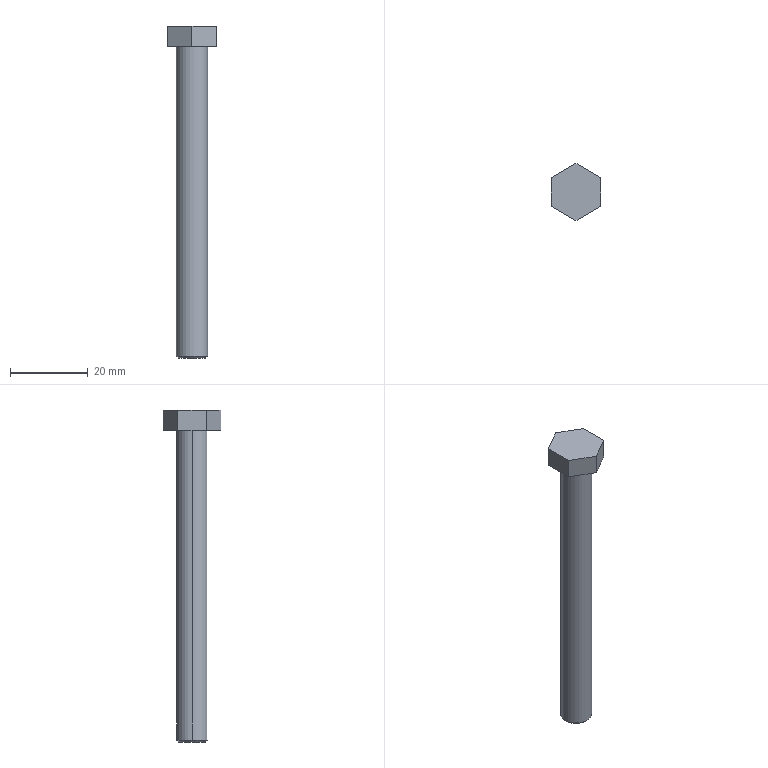Part | STEP file | Bulong M8_8F | 1 solid | 13 faces | box 12.73 x 14.699 x 85.15 mm | volume 4741 mm3 | plane 9 | cone 2 | cylinder 2 | commonest cylinder face diameters 8 x2
STEP:
#1=CARTESIAN_POINT('',(0.,0.,0.));
#2=DIRECTION('',(0.,0.,1.));
#3=DIRECTION('',(1.,0.,0.));
#4=AXIS2_PLACEMENT_3D('',#1,#2,#3);
#5=CARTESIAN_POINT('',(-3.5,0.,-80.));
#6=VERTEX_POINT('',#5);
#7=CARTESIAN_POINT('',(3.5,0.,-80.));
#8=VERTEX_POINT('',#7);
#9=CARTESIAN_POINT('',(0.,0.,-80.));
#10=DIRECTION('',(0.,0.,-1.));
#11=DIRECTION('',(-1.,0.,0.));
#12=AXIS2_PLACEMENT_3D('',#9,#10,#11);
#13=CIRCLE('',#12,3.5);
#14=CARTESIAN_POINT('',(0.,0.,-80.));
#15=DIRECTION('',(0.,0.,1.));
#16=DIRECTION('',(1.,0.,0.));
#17=AXIS2_PLACEMENT_3D('',#14,#15,#16);
#18=CONICAL_SURFACE('',#17,3.5,0.7854);
#19=CARTESIAN_POINT('',(3.142,0.));
#20=DIRECTION('',(-1.,0.));
#21=VECTOR('',#20,1.);
#22=LINE('',#19,#21);
#23=(GEOMETRIC_REPRESENTATION_CONTEXT(2)PARAMETRIC_REPRESENTATION_CONTEXT()REPRESENTATION_CONTEXT('',''));
#24=DEFINITIONAL_REPRESENTATION('',(#22),#23);
#25=PCURVE('',#18,#24);
#26=CARTESIAN_POINT('',(0.,0.,-80.));
#27=DIRECTION('',(0.,0.,-1.));
#28=DIRECTION('',(-1.,0.,0.));
#29=AXIS2_PLACEMENT_3D('',#26,#27,#28);
#30=PLANE('',#29);
#31=CARTESIAN_POINT('',(0.,0.));
#32=DIRECTION('',(1.,0.));
#33=AXIS2_PLACEMENT_2D('',#31,#32);
#34=CIRCLE('',#33,3.5);
#35=(GEOMETRIC_REPRESENTATION_CONTEXT(2)PARAMETRIC_REPRESENTATION_CONTEXT()REPRESENTATION_CONTEXT('',''));
#36=DEFINITIONAL_REPRESENTATION('',(#34),#35);
#37=PCURVE('',#30,#36);
#38=SURFACE_CURVE('',#13,(#25,#37),.PCURVE_S1.);
#39=EDGE_CURVE('',#6,#8,#38,.T.);
#40=ORIENTED_EDGE('',*,*,#39,.F.);
#41=CARTESIAN_POINT('',(-4.,0.,-79.5));
#42=VERTEX_POINT('',#41);
#43=CARTESIAN_POINT('',(-3.5,0.,-80.));
#44=DIRECTION('',(-0.7071,0.,0.7071));
#45=VECTOR('',#44,1.);
#46=LINE('',#43,#45);
#47=CARTESIAN_POINT('',(3.142,0.));
#48=DIRECTION('',(0.,1.));
#49=VECTOR('',#48,1.);
#50=LINE('',#47,#49);
#51=(GEOMETRIC_REPRESENTATION_CONTEXT(2)PARAMETRIC_REPRESENTATION_CONTEXT()REPRESENTATION_CONTEXT('',''));
#52=DEFINITIONAL_REPRESENTATION('',(#50),#51);
#53=PCURVE('',#18,#52);
#54=CARTESIAN_POINT('',(0.,0.,-80.));
#55=DIRECTION('',(0.,0.,1.));
#56=DIRECTION('',(1.,0.,0.));
#57=AXIS2_PLACEMENT_3D('',#54,#55,#56);
#58=CONICAL_SURFACE('',#57,3.5,0.7854);
#59=CARTESIAN_POINT('',(3.142,0.));
#60=DIRECTION('',(0.,1.));
#61=VECTOR('',#60,1.);
#62=LINE('',#59,#61);
#63=(GEOMETRIC_REPRESENTATION_CONTEXT(2)PARAMETRIC_REPRESENTATION_CONTEXT()REPRESENTATION_CONTEXT('',''));
#64=DEFINITIONAL_REPRESENTATION('',(#62),#63);
#65=PCURVE('',#58,#64);
#66=SURFACE_CURVE('',#46,(#53,#65),.PCURVE_S1.);
#67=EDGE_CURVE('',#6,#42,#66,.T.);
#68=ORIENTED_EDGE('',*,*,#67,.T.);
#69=CARTESIAN_POINT('',(4.,0.,-79.5));
#70=VERTEX_POINT('',#69);
#71=CARTESIAN_POINT('',(0.,0.,-79.5));
#72=DIRECTION('',(0.,0.,1.));
#73=DIRECTION('',(-1.,0.,0.));
#74=AXIS2_PLACEMENT_3D('',#71,#72,#73);
#75=CIRCLE('',#74,4.);
#76=CARTESIAN_POINT('',(-3.142,0.5));
#77=DIRECTION('',(1.,0.));
#78=VECTOR('',#77,1.);
#79=LINE('',#76,#78);
#80=(GEOMETRIC_REPRESENTATION_CONTEXT(2)PARAMETRIC_REPRESENTATION_CONTEXT()REPRESENTATION_CONTEXT('',''));
#81=DEFINITIONAL_REPRESENTATION('',(#79),#80);
#82=PCURVE('',#18,#81);
#83=CARTESIAN_POINT('',(0.,0.,-80.));
#84=DIRECTION('',(0.,0.,1.));
#85=DIRECTION('',(1.,0.,0.));
#86=AXIS2_PLACEMENT_3D('',#83,#84,#85);
#87=CYLINDRICAL_SURFACE('',#86,4.);
#88=CARTESIAN_POINT('',(-3.142,0.5));
#89=DIRECTION('',(1.,0.));
#90=VECTOR('',#89,1.);
#91=LINE('',#88,#90);
#92=(GEOMETRIC_REPRESENTATION_CONTEXT(2)PARAMETRIC_REPRESENTATION_CONTEXT()REPRESENTATION_CONTEXT('',''));
#93=DEFINITIONAL_REPRESENTATION('',(#91),#92);
#94=PCURVE('',#87,#93);
#95=SURFACE_CURVE('',#75,(#82,#94),.PCURVE_S1.);
#96=EDGE_CURVE('',#70,#42,#95,.T.);
#97=ORIENTED_EDGE('',*,*,#96,.F.);
#98=CARTESIAN_POINT('',(3.5,0.,-80.));
#99=DIRECTION('',(0.7071,0.,0.7071));
#100=VECTOR('',#99,1.);
#101=LINE('',#98,#100);
#102=CARTESIAN_POINT('',(0.,0.));
#103=DIRECTION('',(0.,1.));
#104=VECTOR('',#103,1.);
#105=LINE('',#102,#104);
#106=(GEOMETRIC_REPRESENTATION_CONTEXT(2)PARAMETRIC_REPRESENTATION_CONTEXT()REPRESENTATION_CONTEXT('',''));
#107=DEFINITIONAL_REPRESENTATION('',(#105),#106);
#108=PCURVE('',#18,#107);
#109=CARTESIAN_POINT('',(6.283,0.));
#110=DIRECTION('',(0.,1.));
#111=VECTOR('',#110,1.);
#112=LINE('',#109,#111);
#113=(GEOMETRIC_REPRESENTATION_CONTEXT(2)PARAMETRIC_REPRESENTATION_CONTEXT()REPRESENTATION_CONTEXT('',''));
#114=DEFINITIONAL_REPRESENTATION('',(#112),#113);
#115=PCURVE('',#58,#114);
#116=SURFACE_CURVE('',#101,(#108,#115),.PCURVE_S1.);
#117=EDGE_CURVE('',#8,#70,#116,.T.);
#118=ORIENTED_EDGE('',*,*,#117,.F.);
#119=EDGE_LOOP('',(#40,#68,#97,#118));
#120=FACE_BOUND('',#119,.T.);
#121=ADVANCED_FACE('',(#120),#18,.T.);
#122=ORIENTED_EDGE('',*,*,#96,.T.);
#123=CARTESIAN_POINT('',(-4.,0.,0.));
#124=VERTEX_POINT('',#123);
#125=CARTESIAN_POINT('',(-4.,0.,-80.));
#126=DIRECTION('',(0.,0.,1.));
#127=VECTOR('',#126,1.);
#128=LINE('',#125,#127);
#129=CARTESIAN_POINT('',(3.142,0.));
#130=DIRECTION('',(0.,1.));
#131=VECTOR('',#130,1.);
#132=LINE('',#129,#131);
#133=(GEOMETRIC_REPRESENTATION_CONTEXT(2)PARAMETRIC_REPRESENTATION_CONTEXT()REPRESENTATION_CONTEXT('',''));
#134=DEFINITIONAL_REPRESENTATION('',(#132),#133);
#135=PCURVE('',#87,#134);
#136=CARTESIAN_POINT('',(0.,0.,-80.));
#137=DIRECTION('',(0.,0.,1.));
#138=DIRECTION('',(1.,0.,0.));
#139=AXIS2_PLACEMENT_3D('',#136,#137,#138);
#140=CYLINDRICAL_SURFACE('',#139,4.);
#141=CARTESIAN_POINT('',(3.142,0.));
#142=DIRECTION('',(0.,1.));
#143=VECTOR('',#142,1.);
#144=LINE('',#141,#143);
#145=(GEOMETRIC_REPRESENTATION_CONTEXT(2)PARAMETRIC_REPRESENTATION_CONTEXT()REPRESENTATION_CONTEXT('',''));
#146=DEFINITIONAL_REPRESENTATION('',(#144),#145);
#147=PCURVE('',#140,#146);
#148=SURFACE_CURVE('',#128,(#135,#147),.PCURVE_S1.);
#149=EDGE_CURVE('',#42,#124,#148,.T.);
#150=ORIENTED_EDGE('',*,*,#149,.T.);
#151=CARTESIAN_POINT('',(4.,0.,0.));
#152=VERTEX_POINT('',#151);
#153=CARTESIAN_POINT('',(0.,0.,0.));
#154=DIRECTION('',(0.,0.,-1.));
#155=DIRECTION('',(1.,0.,0.));
#156=AXIS2_PLACEMENT_3D('',#153,#154,#155);
#157=CIRCLE('',#156,4.);
#158=CARTESIAN_POINT('',(6.283,80.));
#159=DIRECTION('',(-1.,0.));
#160=VECTOR('',#159,1.);
#161=LINE('',#158,#160);
#162=(GEOMETRIC_REPRESENTATION_CONTEXT(2)PARAMETRIC_REPRESENTATION_CONTEXT()REPRESENTATION_CONTEXT('',''));
#163=DEFINITIONAL_REPRESENTATION('',(#161),#162);
#164=PCURVE('',#87,#163);
#165=CARTESIAN_POINT('',(0.,0.,0.));
#166=DIRECTION('',(0.,0.,1.));
#167=DIRECTION('',(1.,0.,0.));
#168=AXIS2_PLACEMENT_3D('',#165,#166,#167);
#169=PLANE('',#168);
#170=CARTESIAN_POINT('',(4.,0.));
#171=CARTESIAN_POINT('',(4.,-6.928));
#172=CARTESIAN_POINT('',(-2.,-3.464));
#173=CARTESIAN_POINT('',(-8.,0.));
#174=CARTESIAN_POINT('',(-2.,3.464));
#175=CARTESIAN_POINT('',(4.,6.928));
#176=CARTESIAN_POINT('',(4.,0.));
#177=(BOUNDED_CURVE()B_SPLINE_CURVE(2,(#170,#171,#172,#173,#174,#175,#176),.UNSPECIFIED.,.T.,.F.)B_SPLINE_CURVE_WITH_KNOTS((1,2,2,2,2,1),(-2.094,0.,2.094,4.189,6.283,8.378),.UNSPECIFIED.)CURVE()GEOMETRIC_REPRESENTATION_ITEM()RATIONAL_B_SPLINE_CURVE((1.,0.5,1.,0.5,1.,0.5,1.))REPRESENTATION_ITEM(''));
#178=(GEOMETRIC_REPRESENTATION_CONTEXT(2)PARAMETRIC_REPRESENTATION_CONTEXT()REPRESENTATION_CONTEXT('',''));
#179=DEFINITIONAL_REPRESENTATION('',(#177),#178);
#180=PCURVE('',#169,#179);
#181=SURFACE_CURVE('',#157,(#164,#180),.PCURVE_S1.);
#182=EDGE_CURVE('',#124,#152,#181,.T.);
#183=ORIENTED_EDGE('',*,*,#182,.T.);
#184=CARTESIAN_POINT('',(4.,0.,-80.));
#185=DIRECTION('',(0.,0.,1.));
#186=VECTOR('',#185,1.);
#187=LINE('',#184,#186);
#188=CARTESIAN_POINT('',(0.,0.));
#189=DIRECTION('',(0.,1.));
#190=VECTOR('',#189,1.);
#191=LINE('',#188,#190);
#192=(GEOMETRIC_REPRESENTATION_CONTEXT(2)PARAMETRIC_REPRESENTATION_CONTEXT()REPRESENTATION_CONTEXT('',''));
#193=DEFINITIONAL_REPRESENTATION('',(#191),#192);
#194=PCURVE('',#87,#193);
#195=CARTESIAN_POINT('',(6.283,0.));
#196=DIRECTION('',(0.,1.));
#197=VECTOR('',#196,1.);
#198=LINE('',#195,#197);
#199=(GEOMETRIC_REPRESENTATION_CONTEXT(2)PARAMETRIC_REPRESENTATION_CONTEXT()REPRESENTATION_CONTEXT('',''));
#200=DEFINITIONAL_REPRESENTATION('',(#198),#199);
#201=PCURVE('',#140,#200);
#202=SURFACE_CURVE('',#187,(#194,#201),.PCURVE_S1.);
#203=EDGE_CURVE('',#70,#152,#202,.T.);
#204=ORIENTED_EDGE('',*,*,#203,.F.);
#205=EDGE_LOOP('',(#122,#150,#183,#204));
#206=FACE_BOUND('',#205,.T.);
#207=ADVANCED_FACE('',(#206),#87,.T.);
#208=CARTESIAN_POINT('',(6.365,3.675,0.));
#209=VERTEX_POINT('',#208);
#210=CARTESIAN_POINT('',(0.,7.35,0.));
#211=VERTEX_POINT('',#210);
#212=CARTESIAN_POINT('',(6.365,3.675,0.));
#213=DIRECTION('',(-0.866,0.5,0.));
#214=VECTOR('',#213,1.);
#215=LINE('',#212,#214);
#216=CARTESIAN_POINT('',(6.365,3.675));
#217=DIRECTION('',(-0.866,0.5));
#218=VECTOR('',#217,1.);
#219=LINE('',#216,#218);
#220=(GEOMETRIC_REPRESENTATION_CONTEXT(2)PARAMETRIC_REPRESENTATION_CONTEXT()REPRESENTATION_CONTEXT('',''));
#221=DEFINITIONAL_REPRESENTATION('',(#219),#220);
#222=PCURVE('',#169,#221);
#223=CARTESIAN_POINT('',(6.365,3.675,5.15));
#224=DIRECTION('',(-0.5,-0.866,0.));
#225=DIRECTION('',(0.866,-0.5,0.));
#226=AXIS2_PLACEMENT_3D('',#223,#224,#225);
#227=PLANE('',#226);
#228=CARTESIAN_POINT('',(0.,-5.15));
#229=DIRECTION('',(-1.,0.));
#230=VECTOR('',#229,1.);
#231=LINE('',#228,#230);
#232=(GEOMETRIC_REPRESENTATION_CONTEXT(2)PARAMETRIC_REPRESENTATION_CONTEXT()REPRESENTATION_CONTEXT('',''));
#233=DEFINITIONAL_REPRESENTATION('',(#231),#232);
#234=PCURVE('',#227,#233);
#235=SURFACE_CURVE('',#215,(#222,#234),.PCURVE_S1.);
#236=EDGE_CURVE('',#209,#211,#235,.T.);
#237=ORIENTED_EDGE('',*,*,#236,.F.);
#238=CARTESIAN_POINT('',(6.365,-3.675,0.));
#239=VERTEX_POINT('',#238);
#240=CARTESIAN_POINT('',(6.365,-3.675,0.));
#241=DIRECTION('',(0.,1.,0.));
#242=VECTOR('',#241,1.);
#243=LINE('',#240,#242);
#244=CARTESIAN_POINT('',(6.365,-3.675));
#245=DIRECTION('',(0.,1.));
#246=VECTOR('',#245,1.);
#247=LINE('',#244,#246);
#248=(GEOMETRIC_REPRESENTATION_CONTEXT(2)PARAMETRIC_REPRESENTATION_CONTEXT()REPRESENTATION_CONTEXT('',''));
#249=DEFINITIONAL_REPRESENTATION('',(#247),#248);
#250=PCURVE('',#169,#249);
#251=CARTESIAN_POINT('',(6.365,-3.675,5.15));
#252=DIRECTION('',(-1.,0.,0.));
#253=DIRECTION('',(0.,-1.,0.));
#254=AXIS2_PLACEMENT_3D('',#251,#252,#253);
#255=PLANE('',#254);
#256=CARTESIAN_POINT('',(0.,-5.15));
#257=DIRECTION('',(-1.,0.));
#258=VECTOR('',#257,1.);
#259=LINE('',#256,#258);
#260=(GEOMETRIC_REPRESENTATION_CONTEXT(2)PARAMETRIC_REPRESENTATION_CONTEXT()REPRESENTATION_CONTEXT('',''));
#261=DEFINITIONAL_REPRESENTATION('',(#259),#260);
#262=PCURVE('',#255,#261);
#263=SURFACE_CURVE('',#243,(#250,#262),.PCURVE_S1.);
#264=EDGE_CURVE('',#239,#209,#263,.T.);
#265=ORIENTED_EDGE('',*,*,#264,.F.);
#266=CARTESIAN_POINT('',(0.,-7.35,0.));
#267=VERTEX_POINT('',#266);
#268=CARTESIAN_POINT('',(0.,-7.35,0.));
#269=DIRECTION('',(0.866,0.5,0.));
#270=VECTOR('',#269,1.);
#271=LINE('',#268,#270);
#272=CARTESIAN_POINT('',(0.,-7.35));
#273=DIRECTION('',(0.866,0.5));
#274=VECTOR('',#273,1.);
#275=LINE('',#272,#274);
#276=(GEOMETRIC_REPRESENTATION_CONTEXT(2)PARAMETRIC_REPRESENTATION_CONTEXT()REPRESENTATION_CONTEXT('',''));
#277=DEFINITIONAL_REPRESENTATION('',(#275),#276);
#278=PCURVE('',#169,#277);
#279=CARTESIAN_POINT('',(0.,-7.35,5.15));
#280=DIRECTION('',(-0.5,0.866,0.));
#281=DIRECTION('',(-0.866,-0.5,0.));
#282=AXIS2_PLACEMENT_3D('',#279,#280,#281);
#283=PLANE('',#282);
#284=CARTESIAN_POINT('',(0.,-5.15));
#285=DIRECTION('',(-1.,0.));
#286=VECTOR('',#285,1.);
#287=LINE('',#284,#286);
#288=(GEOMETRIC_REPRESENTATION_CONTEXT(2)PARAMETRIC_REPRESENTATION_CONTEXT()REPRESENTATION_CONTEXT('',''));
#289=DEFINITIONAL_REPRESENTATION('',(#287),#288);
#290=PCURVE('',#283,#289);
#291=SURFACE_CURVE('',#271,(#278,#290),.PCURVE_S1.);
#292=EDGE_CURVE('',#267,#239,#291,.T.);
#293=ORIENTED_EDGE('',*,*,#292,.F.);
#294=CARTESIAN_POINT('',(-6.365,-3.675,0.));
#295=VERTEX_POINT('',#294);
#296=CARTESIAN_POINT('',(-6.365,-3.675,0.));
#297=DIRECTION('',(0.866,-0.5,0.));
#298=VECTOR('',#297,1.);
#299=LINE('',#296,#298);
#300=CARTESIAN_POINT('',(-6.365,-3.675));
#301=DIRECTION('',(0.866,-0.5));
#302=VECTOR('',#301,1.);
#303=LINE('',#300,#302);
#304=(GEOMETRIC_REPRESENTATION_CONTEXT(2)PARAMETRIC_REPRESENTATION_CONTEXT()REPRESENTATION_CONTEXT('',''));
#305=DEFINITIONAL_REPRESENTATION('',(#303),#304);
#306=PCURVE('',#169,#305);
#307=CARTESIAN_POINT('',(-6.365,-3.675,5.15));
#308=DIRECTION('',(0.5,0.866,0.));
#309=DIRECTION('',(-0.866,0.5,0.));
#310=AXIS2_PLACEMENT_3D('',#307,#308,#309);
#311=PLANE('',#310);
#312=CARTESIAN_POINT('',(0.,-5.15));
#313=DIRECTION('',(-1.,0.));
#314=VECTOR('',#313,1.);
#315=LINE('',#312,#314);
#316=(GEOMETRIC_REPRESENTATION_CONTEXT(2)PARAMETRIC_REPRESENTATION_CONTEXT()REPRESENTATION_CONTEXT('',''));
#317=DEFINITIONAL_REPRESENTATION('',(#315),#316);
#318=PCURVE('',#311,#317);
#319=SURFACE_CURVE('',#299,(#306,#318),.PCURVE_S1.);
#320=EDGE_CURVE('',#295,#267,#319,.T.);
#321=ORIENTED_EDGE('',*,*,#320,.F.);
#322=CARTESIAN_POINT('',(-6.365,3.675,0.));
#323=VERTEX_POINT('',#322);
#324=CARTESIAN_POINT('',(-6.365,3.675,0.));
#325=DIRECTION('',(0.,-1.,0.));
#326=VECTOR('',#325,1.);
#327=LINE('',#324,#326);
#328=CARTESIAN_POINT('',(-6.365,3.675));
#329=DIRECTION('',(0.,-1.));
#330=VECTOR('',#329,1.);
#331=LINE('',#328,#330);
#332=(GEOMETRIC_REPRESENTATION_CONTEXT(2)PARAMETRIC_REPRESENTATION_CONTEXT()REPRESENTATION_CONTEXT('',''));
#333=DEFINITIONAL_REPRESENTATION('',(#331),#332);
#334=PCURVE('',#169,#333);
#335=CARTESIAN_POINT('',(-6.365,3.675,5.15));
#336=DIRECTION('',(1.,0.,0.));
#337=DIRECTION('',(0.,0.,-1.));
#338=AXIS2_PLACEMENT_3D('',#335,#336,#337);
#339=PLANE('',#338);
#340=CARTESIAN_POINT('',(5.15,0.));
#341=DIRECTION('',(0.,-1.));
#342=VECTOR('',#341,1.);
#343=LINE('',#340,#342);
#344=(GEOMETRIC_REPRESENTATION_CONTEXT(2)PARAMETRIC_REPRESENTATION_CONTEXT()REPRESENTATION_CONTEXT('',''));
#345=DEFINITIONAL_REPRESENTATION('',(#343),#344);
#346=PCURVE('',#339,#345);
#347=SURFACE_CURVE('',#327,(#334,#346),.PCURVE_S1.);
#348=EDGE_CURVE('',#323,#295,#347,.T.);
#349=ORIENTED_EDGE('',*,*,#348,.F.);
#350=CARTESIAN_POINT('',(0.,7.35,0.));
#351=DIRECTION('',(-0.866,-0.5,0.));
#352=VECTOR('',#351,1.);
#353=LINE('',#350,#352);
#354=CARTESIAN_POINT('',(0.,7.35));
#355=DIRECTION('',(-0.866,-0.5));
#356=VECTOR('',#355,1.);
#357=LINE('',#354,#356);
#358=(GEOMETRIC_REPRESENTATION_CONTEXT(2)PARAMETRIC_REPRESENTATION_CONTEXT()REPRESENTATION_CONTEXT('',''));
#359=DEFINITIONAL_REPRESENTATION('',(#357),#358);
#360=PCURVE('',#169,#359);
#361=CARTESIAN_POINT('',(0.,7.35,5.15));
#362=DIRECTION('',(0.5,-0.866,0.));
#363=DIRECTION('',(0.866,0.5,0.));
#364=AXIS2_PLACEMENT_3D('',#361,#362,#363);
#365=PLANE('',#364);
#366=CARTESIAN_POINT('',(0.,-5.15));
#367=DIRECTION('',(-1.,0.));
#368=VECTOR('',#367,1.);
#369=LINE('',#366,#368);
#370=(GEOMETRIC_REPRESENTATION_CONTEXT(2)PARAMETRIC_REPRESENTATION_CONTEXT()REPRESENTATION_CONTEXT('',''));
#371=DEFINITIONAL_REPRESENTATION('',(#369),#370);
#372=PCURVE('',#365,#371);
#373=SURFACE_CURVE('',#353,(#360,#372),.PCURVE_S1.);
#374=EDGE_CURVE('',#211,#323,#373,.T.);
#375=ORIENTED_EDGE('',*,*,#374,.F.);
#376=EDGE_LOOP('',(#237,#265,#293,#321,#349,#375));
#377=FACE_BOUND('',#376,.T.);
#378=CARTESIAN_POINT('',(0.,0.,0.));
#379=DIRECTION('',(0.,0.,-1.));
#380=DIRECTION('',(1.,0.,0.));
#381=AXIS2_PLACEMENT_3D('',#378,#379,#380);
#382=CIRCLE('',#381,4.);
#383=CARTESIAN_POINT('',(4.,0.));
#384=CARTESIAN_POINT('',(4.,-6.928));
#385=CARTESIAN_POINT('',(-2.,-3.464));
#386=CARTESIAN_POINT('',(-8.,0.));
#387=CARTESIAN_POINT('',(-2.,3.464));
#388=CARTESIAN_POINT('',(4.,6.928));
#389=CARTESIAN_POINT('',(4.,0.));
#390=(BOUNDED_CURVE()B_SPLINE_CURVE(2,(#383,#384,#385,#386,#387,#388,#389),.UNSPECIFIED.,.T.,.F.)B_SPLINE_CURVE_WITH_KNOTS((1,2,2,2,2,1),(-2.094,0.,2.094,4.189,6.283,8.378),.UNSPECIFIED.)CURVE()GEOMETRIC_REPRESENTATION_ITEM()RATIONAL_B_SPLINE_CURVE((1.,0.5,1.,0.5,1.,0.5,1.))REPRESENTATION_ITEM(''));
#391=(GEOMETRIC_REPRESENTATION_CONTEXT(2)PARAMETRIC_REPRESENTATION_CONTEXT()REPRESENTATION_CONTEXT('',''));
#392=DEFINITIONAL_REPRESENTATION('',(#390),#391);
#393=PCURVE('',#169,#392);
#394=CARTESIAN_POINT('',(6.283,80.));
#395=DIRECTION('',(-1.,0.));
#396=VECTOR('',#395,1.);
#397=LINE('',#394,#396);
#398=(GEOMETRIC_REPRESENTATION_CONTEXT(2)PARAMETRIC_REPRESENTATION_CONTEXT()REPRESENTATION_CONTEXT('',''));
#399=DEFINITIONAL_REPRESENTATION('',(#397),#398);
#400=PCURVE('',#140,#399);
#401=SURFACE_CURVE('',#382,(#393,#400),.PCURVE_S1.);
#402=EDGE_CURVE('',#152,#124,#401,.T.);
#403=ORIENTED_EDGE('',*,*,#402,.F.);
#404=ORIENTED_EDGE('',*,*,#182,.F.);
#405=EDGE_LOOP('',(#403,#404));
#406=FACE_BOUND('',#405,.T.);
#407=ADVANCED_FACE('',(#377,#406),#169,.F.);
#408=ORIENTED_EDGE('',*,*,#236,.T.);
#409=CARTESIAN_POINT('',(0.,7.35,5.15));
#410=VERTEX_POINT('',#409);
#411=CARTESIAN_POINT('',(0.,7.35,5.15));
#412=DIRECTION('',(0.,0.,-1.));
#413=VECTOR('',#412,1.);
#414=LINE('',#411,#413);
#415=CARTESIAN_POINT('',(-7.35,0.));
#416=DIRECTION('',(0.,-1.));
#417=VECTOR('',#416,1.);
#418=LINE('',#415,#417);
#419=(GEOMETRIC_REPRESENTATION_CONTEXT(2)PARAMETRIC_REPRESENTATION_CONTEXT()REPRESENTATION_CONTEXT('',''));
#420=DEFINITIONAL_REPRESENTATION('',(#418),#419);
#421=PCURVE('',#227,#420);
#422=CARTESIAN_POINT('',(0.,0.));
#423=DIRECTION('',(0.,-1.));
#424=VECTOR('',#423,1.);
#425=LINE('',#422,#424);
#426=(GEOMETRIC_REPRESENTATION_CONTEXT(2)PARAMETRIC_REPRESENTATION_CONTEXT()REPRESENTATION_CONTEXT('',''));
#427=DEFINITIONAL_REPRESENTATION('',(#425),#426);
#428=PCURVE('',#365,#427);
#429=SURFACE_CURVE('',#414,(#421,#428),.PCURVE_S1.);
#430=EDGE_CURVE('',#410,#211,#429,.T.);
#431=ORIENTED_EDGE('',*,*,#430,.F.);
#432=CARTESIAN_POINT('',(6.365,3.675,5.15));
#433=VERTEX_POINT('',#432);
#434=CARTESIAN_POINT('',(6.365,3.675,5.15));
#435=DIRECTION('',(-0.866,0.5,0.));
#436=VECTOR('',#435,1.);
#437=LINE('',#434,#436);
#438=CARTESIAN_POINT('',(0.,0.));
#439=DIRECTION('',(-1.,0.));
#440=VECTOR('',#439,1.);
#441=LINE('',#438,#440);
#442=(GEOMETRIC_REPRESENTATION_CONTEXT(2)PARAMETRIC_REPRESENTATION_CONTEXT()REPRESENTATION_CONTEXT('',''));
#443=DEFINITIONAL_REPRESENTATION('',(#441),#442);
#444=PCURVE('',#227,#443);
#445=CARTESIAN_POINT('',(0.,0.,5.15));
#446=DIRECTION('',(0.,0.,1.));
#447=DIRECTION('',(1.,0.,0.));
#448=AXIS2_PLACEMENT_3D('',#445,#446,#447);
#449=PLANE('',#448);
#450=CARTESIAN_POINT('',(6.365,3.675));
#451=DIRECTION('',(-0.866,0.5));
#452=VECTOR('',#451,1.);
#453=LINE('',#450,#452);
#454=(GEOMETRIC_REPRESENTATION_CONTEXT(2)PARAMETRIC_REPRESENTATION_CONTEXT()REPRESENTATION_CONTEXT('',''));
#455=DEFINITIONAL_REPRESENTATION('',(#453),#454);
#456=PCURVE('',#449,#455);
#457=SURFACE_CURVE('',#437,(#444,#456),.PCURVE_S1.);
#458=EDGE_CURVE('',#433,#410,#457,.T.);
#459=ORIENTED_EDGE('',*,*,#458,.F.);
#460=CARTESIAN_POINT('',(6.365,3.675,5.15));
#461=DIRECTION('',(0.,0.,-1.));
#462=VECTOR('',#461,1.);
#463=LINE('',#460,#462);
#464=CARTESIAN_POINT('',(0.,0.));
#465=DIRECTION('',(0.,-1.));
#466=VECTOR('',#465,1.);
#467=LINE('',#464,#466);
#468=(GEOMETRIC_REPRESENTATION_CONTEXT(2)PARAMETRIC_REPRESENTATION_CONTEXT()REPRESENTATION_CONTEXT('',''));
#469=DEFINITIONAL_REPRESENTATION('',(#467),#468);
#470=PCURVE('',#227,#469);
#471=CARTESIAN_POINT('',(-7.35,0.));
#472=DIRECTION('',(0.,-1.));
#473=VECTOR('',#472,1.);
#474=LINE('',#471,#473);
#475=(GEOMETRIC_REPRESENTATION_CONTEXT(2)PARAMETRIC_REPRESENTATION_CONTEXT()REPRESENTATION_CONTEXT('',''));
#476=DEFINITIONAL_REPRESENTATION('',(#474),#475);
#477=PCURVE('',#255,#476);
#478=SURFACE_CURVE('',#463,(#470,#477),.PCURVE_S1.);
#479=EDGE_CURVE('',#433,#209,#478,.T.);
#480=ORIENTED_EDGE('',*,*,#479,.T.);
#481=EDGE_LOOP('',(#408,#431,#459,#480));
#482=FACE_BOUND('',#481,.T.);
#483=ADVANCED_FACE('',(#482),#227,.F.);
#484=ORIENTED_EDGE('',*,*,#374,.T.);
#485=CARTESIAN_POINT('',(-6.365,3.675,5.15));
#486=VERTEX_POINT('',#485);
#487=CARTESIAN_POINT('',(-6.365,3.675,5.15));
#488=DIRECTION('',(0.,0.,-1.));
#489=VECTOR('',#488,1.);
#490=LINE('',#487,#489);
#491=CARTESIAN_POINT('',(-7.35,0.));
#492=DIRECTION('',(0.,-1.));
#493=VECTOR('',#492,1.);
#494=LINE('',#491,#493);
#495=(GEOMETRIC_REPRESENTATION_CONTEXT(2)PARAMETRIC_REPRESENTATION_CONTEXT()REPRESENTATION_CONTEXT('',''));
#496=DEFINITIONAL_REPRESENTATION('',(#494),#495);
#497=PCURVE('',#365,#496);
#498=CARTESIAN_POINT('',(0.,0.));
#499=DIRECTION('',(1.,0.));
#500=VECTOR('',#499,1.);
#501=LINE('',#498,#500);
#502=(GEOMETRIC_REPRESENTATION_CONTEXT(2)PARAMETRIC_REPRESENTATION_CONTEXT()REPRESENTATION_CONTEXT('',''));
#503=DEFINITIONAL_REPRESENTATION('',(#501),#502);
#504=PCURVE('',#339,#503);
#505=SURFACE_CURVE('',#490,(#497,#504),.PCURVE_S1.);
#506=EDGE_CURVE('',#486,#323,#505,.T.);
#507=ORIENTED_EDGE('',*,*,#506,.F.);
#508=CARTESIAN_POINT('',(0.,7.35,5.15));
#509=DIRECTION('',(-0.866,-0.5,0.));
#510=VECTOR('',#509,1.);
#511=LINE('',#508,#510);
#512=CARTESIAN_POINT('',(0.,0.));
#513=DIRECTION('',(-1.,0.));
#514=VECTOR('',#513,1.);
#515=LINE('',#512,#514);
#516=(GEOMETRIC_REPRESENTATION_CONTEXT(2)PARAMETRIC_REPRESENTATION_CONTEXT()REPRESENTATION_CONTEXT('',''));
#517=DEFINITIONAL_REPRESENTATION('',(#515),#516);
#518=PCURVE('',#365,#517);
#519=CARTESIAN_POINT('',(0.,7.35));
#520=DIRECTION('',(-0.866,-0.5));
#521=VECTOR('',#520,1.);
#522=LINE('',#519,#521);
#523=(GEOMETRIC_REPRESENTATION_CONTEXT(2)PARAMETRIC_REPRESENTATION_CONTEXT()REPRESENTATION_CONTEXT('',''));
#524=DEFINITIONAL_REPRESENTATION('',(#522),#523);
#525=PCURVE('',#449,#524);
#526=SURFACE_CURVE('',#511,(#518,#525),.PCURVE_S1.);
#527=EDGE_CURVE('',#410,#486,#526,.T.);
#528=ORIENTED_EDGE('',*,*,#527,.F.);
#529=ORIENTED_EDGE('',*,*,#430,.T.);
#530=EDGE_LOOP('',(#484,#507,#528,#529));
#531=FACE_BOUND('',#530,.T.);
#532=ADVANCED_FACE('',(#531),#365,.F.);
#533=ORIENTED_EDGE('',*,*,#348,.T.);
#534=CARTESIAN_POINT('',(-6.365,-3.675,5.15));
#535=VERTEX_POINT('',#534);
#536=CARTESIAN_POINT('',(-6.365,-3.675,5.15));
#537=DIRECTION('',(0.,0.,-1.));
#538=VECTOR('',#537,1.);
#539=LINE('',#536,#538);
#540=CARTESIAN_POINT('',(0.,-7.35));
#541=DIRECTION('',(1.,0.));
#542=VECTOR('',#541,1.);
#543=LINE('',#540,#542);
#544=(GEOMETRIC_REPRESENTATION_CONTEXT(2)PARAMETRIC_REPRESENTATION_CONTEXT()REPRESENTATION_CONTEXT('',''));
#545=DEFINITIONAL_REPRESENTATION('',(#543),#544);
#546=PCURVE('',#339,#545);
#547=CARTESIAN_POINT('',(0.,0.));
#548=DIRECTION('',(0.,-1.));
#549=VECTOR('',#548,1.);
#550=LINE('',#547,#549);
#551=(GEOMETRIC_REPRESENTATION_CONTEXT(2)PARAMETRIC_REPRESENTATION_CONTEXT()REPRESENTATION_CONTEXT('',''));
#552=DEFINITIONAL_REPRESENTATION('',(#550),#551);
#553=PCURVE('',#311,#552);
#554=SURFACE_CURVE('',#539,(#546,#553),.PCURVE_S1.);
#555=EDGE_CURVE('',#535,#295,#554,.T.);
#556=ORIENTED_EDGE('',*,*,#555,.F.);
#557=CARTESIAN_POINT('',(-6.365,3.675,5.15));
#558=DIRECTION('',(0.,-1.,0.));
#559=VECTOR('',#558,1.);
#560=LINE('',#557,#559);
#561=CARTESIAN_POINT('',(0.,0.));
#562=DIRECTION('',(0.,-1.));
#563=VECTOR('',#562,1.);
#564=LINE('',#561,#563);
#565=(GEOMETRIC_REPRESENTATION_CONTEXT(2)PARAMETRIC_REPRESENTATION_CONTEXT()REPRESENTATION_CONTEXT('',''));
#566=DEFINITIONAL_REPRESENTATION('',(#564),#565);
#567=PCURVE('',#339,#566);
#568=CARTESIAN_POINT('',(-6.365,3.675));
#569=DIRECTION('',(0.,-1.));
#570=VECTOR('',#569,1.);
#571=LINE('',#568,#570);
#572=(GEOMETRIC_REPRESENTATION_CONTEXT(2)PARAMETRIC_REPRESENTATION_CONTEXT()REPRESENTATION_CONTEXT('',''));
#573=DEFINITIONAL_REPRESENTATION('',(#571),#572);
#574=PCURVE('',#449,#573);
#575=SURFACE_CURVE('',#560,(#567,#574),.PCURVE_S1.);
#576=EDGE_CURVE('',#486,#535,#575,.T.);
#577=ORIENTED_EDGE('',*,*,#576,.F.);
#578=ORIENTED_EDGE('',*,*,#506,.T.);
#579=EDGE_LOOP('',(#533,#556,#577,#578));
#580=FACE_BOUND('',#579,.T.);
#581=ADVANCED_FACE('',(#580),#339,.F.);
#582=ORIENTED_EDGE('',*,*,#320,.T.);
#583=CARTESIAN_POINT('',(0.,-7.35,5.15));
#584=VERTEX_POINT('',#583);
#585=CARTESIAN_POINT('',(0.,-7.35,5.15));
#586=DIRECTION('',(0.,0.,-1.));
#587=VECTOR('',#586,1.);
#588=LINE('',#585,#587);
#589=CARTESIAN_POINT('',(-7.35,0.));
#590=DIRECTION('',(0.,-1.));
#591=VECTOR('',#590,1.);
#592=LINE('',#589,#591);
#593=(GEOMETRIC_REPRESENTATION_CONTEXT(2)PARAMETRIC_REPRESENTATION_CONTEXT()REPRESENTATION_CONTEXT('',''));
#594=DEFINITIONAL_REPRESENTATION('',(#592),#593);
#595=PCURVE('',#311,#594);
#596=CARTESIAN_POINT('',(0.,0.));
#597=DIRECTION('',(0.,-1.));
#598=VECTOR('',#597,1.);
#599=LINE('',#596,#598);
#600=(GEOMETRIC_REPRESENTATION_CONTEXT(2)PARAMETRIC_REPRESENTATION_CONTEXT()REPRESENTATION_CONTEXT('',''));
#601=DEFINITIONAL_REPRESENTATION('',(#599),#600);
#602=PCURVE('',#283,#601);
#603=SURFACE_CURVE('',#588,(#595,#602),.PCURVE_S1.);
#604=EDGE_CURVE('',#584,#267,#603,.T.);
#605=ORIENTED_EDGE('',*,*,#604,.F.);
#606=CARTESIAN_POINT('',(-6.365,-3.675,5.15));
#607=DIRECTION('',(0.866,-0.5,0.));
#608=VECTOR('',#607,1.);
#609=LINE('',#606,#608);
#610=CARTESIAN_POINT('',(0.,0.));
#611=DIRECTION('',(-1.,0.));
#612=VECTOR('',#611,1.);
#613=LINE('',#610,#612);
#614=(GEOMETRIC_REPRESENTATION_CONTEXT(2)PARAMETRIC_REPRESENTATION_CONTEXT()REPRESENTATION_CONTEXT('',''));
#615=DEFINITIONAL_REPRESENTATION('',(#613),#614);
#616=PCURVE('',#311,#615);
#617=CARTESIAN_POINT('',(-6.365,-3.675));
#618=DIRECTION('',(0.866,-0.5));
#619=VECTOR('',#618,1.);
#620=LINE('',#617,#619);
#621=(GEOMETRIC_REPRESENTATION_CONTEXT(2)PARAMETRIC_REPRESENTATION_CONTEXT()REPRESENTATION_CONTEXT('',''));
#622=DEFINITIONAL_REPRESENTATION('',(#620),#621);
#623=PCURVE('',#449,#622);
#624=SURFACE_CURVE('',#609,(#616,#623),.PCURVE_S1.);
#625=EDGE_CURVE('',#535,#584,#624,.T.);
#626=ORIENTED_EDGE('',*,*,#625,.F.);
#627=ORIENTED_EDGE('',*,*,#555,.T.);
#628=EDGE_LOOP('',(#582,#605,#626,#627));
#629=FACE_BOUND('',#628,.T.);
#630=ADVANCED_FACE('',(#629),#311,.F.);
#631=ORIENTED_EDGE('',*,*,#292,.T.);
#632=CARTESIAN_POINT('',(6.365,-3.675,5.15));
#633=VERTEX_POINT('',#632);
#634=CARTESIAN_POINT('',(6.365,-3.675,5.15));
#635=DIRECTION('',(0.,0.,-1.));
#636=VECTOR('',#635,1.);
#637=LINE('',#634,#636);
#638=CARTESIAN_POINT('',(-7.35,0.));
#639=DIRECTION('',(0.,-1.));
#640=VECTOR('',#639,1.);
#641=LINE('',#638,#640);
#642=(GEOMETRIC_REPRESENTATION_CONTEXT(2)PARAMETRIC_REPRESENTATION_CONTEXT()REPRESENTATION_CONTEXT('',''));
#643=DEFINITIONAL_REPRESENTATION('',(#641),#642);
#644=PCURVE('',#283,#643);
#645=CARTESIAN_POINT('',(0.,0.));
#646=DIRECTION('',(0.,-1.));
#647=VECTOR('',#646,1.);
#648=LINE('',#645,#647);
#649=(GEOMETRIC_REPRESENTATION_CONTEXT(2)PARAMETRIC_REPRESENTATION_CONTEXT()REPRESENTATION_CONTEXT('',''));
#650=DEFINITIONAL_REPRESENTATION('',(#648),#649);
#651=PCURVE('',#255,#650);
#652=SURFACE_CURVE('',#637,(#644,#651),.PCURVE_S1.);
#653=EDGE_CURVE('',#633,#239,#652,.T.);
#654=ORIENTED_EDGE('',*,*,#653,.F.);
#655=CARTESIAN_POINT('',(0.,-7.35,5.15));
#656=DIRECTION('',(0.866,0.5,0.));
#657=VECTOR('',#656,1.);
#658=LINE('',#655,#657);
#659=CARTESIAN_POINT('',(0.,0.));
#660=DIRECTION('',(-1.,0.));
#661=VECTOR('',#660,1.);
#662=LINE('',#659,#661);
#663=(GEOMETRIC_REPRESENTATION_CONTEXT(2)PARAMETRIC_REPRESENTATION_CONTEXT()REPRESENTATION_CONTEXT('',''));
#664=DEFINITIONAL_REPRESENTATION('',(#662),#663);
#665=PCURVE('',#283,#664);
#666=CARTESIAN_POINT('',(0.,-7.35));
#667=DIRECTION('',(0.866,0.5));
#668=VECTOR('',#667,1.);
#669=LINE('',#666,#668);
#670=(GEOMETRIC_REPRESENTATION_CONTEXT(2)PARAMETRIC_REPRESENTATION_CONTEXT()REPRESENTATION_CONTEXT('',''));
#671=DEFINITIONAL_REPRESENTATION('',(#669),#670);
#672=PCURVE('',#449,#671);
#673=SURFACE_CURVE('',#658,(#665,#672),.PCURVE_S1.);
#674=EDGE_CURVE('',#584,#633,#673,.T.);
#675=ORIENTED_EDGE('',*,*,#674,.F.);
#676=ORIENTED_EDGE('',*,*,#604,.T.);
#677=EDGE_LOOP('',(#631,#654,#675,#676));
#678=FACE_BOUND('',#677,.T.);
#679=ADVANCED_FACE('',(#678),#283,.F.);
#680=ORIENTED_EDGE('',*,*,#264,.T.);
#681=ORIENTED_EDGE('',*,*,#479,.F.);
#682=CARTESIAN_POINT('',(6.365,-3.675,5.15));
#683=DIRECTION('',(0.,1.,0.));
#684=VECTOR('',#683,1.);
#685=LINE('',#682,#684);
#686=CARTESIAN_POINT('',(0.,0.));
#687=DIRECTION('',(-1.,0.));
#688=VECTOR('',#687,1.);
#689=LINE('',#686,#688);
#690=(GEOMETRIC_REPRESENTATION_CONTEXT(2)PARAMETRIC_REPRESENTATION_CONTEXT()REPRESENTATION_CONTEXT('',''));
#691=DEFINITIONAL_REPRESENTATION('',(#689),#690);
#692=PCURVE('',#255,#691);
#693=CARTESIAN_POINT('',(6.365,-3.675));
#694=DIRECTION('',(0.,1.));
#695=VECTOR('',#694,1.);
#696=LINE('',#693,#695);
#697=(GEOMETRIC_REPRESENTATION_CONTEXT(2)PARAMETRIC_REPRESENTATION_CONTEXT()REPRESENTATION_CONTEXT('',''));
#698=DEFINITIONAL_REPRESENTATION('',(#696),#697);
#699=PCURVE('',#449,#698);
#700=SURFACE_CURVE('',#685,(#692,#699),.PCURVE_S1.);
#701=EDGE_CURVE('',#633,#433,#700,.T.);
#702=ORIENTED_EDGE('',*,*,#701,.F.);
#703=ORIENTED_EDGE('',*,*,#653,.T.);
#704=EDGE_LOOP('',(#680,#681,#702,#703));
#705=FACE_BOUND('',#704,.T.);
#706=ADVANCED_FACE('',(#705),#255,.F.);
#707=ORIENTED_EDGE('',*,*,#458,.T.);
#708=ORIENTED_EDGE('',*,*,#527,.T.);
#709=ORIENTED_EDGE('',*,*,#576,.T.);
#710=ORIENTED_EDGE('',*,*,#625,.T.);
#711=ORIENTED_EDGE('',*,*,#674,.T.);
#712=ORIENTED_EDGE('',*,*,#701,.T.);
#713=EDGE_LOOP('',(#707,#708,#709,#710,#711,#712));
#714=FACE_BOUND('',#713,.T.);
#715=ADVANCED_FACE('',(#714),#449,.T.);
#716=ORIENTED_EDGE('',*,*,#149,.F.);
#717=CARTESIAN_POINT('',(0.,0.,-79.5));
#718=DIRECTION('',(0.,0.,1.));
#719=DIRECTION('',(-1.,0.,0.));
#720=AXIS2_PLACEMENT_3D('',#717,#718,#719);
#721=CIRCLE('',#720,4.);
#722=CARTESIAN_POINT('',(3.142,0.5));
#723=DIRECTION('',(1.,0.));
#724=VECTOR('',#723,1.);
#725=LINE('',#722,#724);
#726=(GEOMETRIC_REPRESENTATION_CONTEXT(2)PARAMETRIC_REPRESENTATION_CONTEXT()REPRESENTATION_CONTEXT('',''));
#727=DEFINITIONAL_REPRESENTATION('',(#725),#726);
#728=PCURVE('',#140,#727);
#729=CARTESIAN_POINT('',(3.142,0.5));
#730=DIRECTION('',(1.,0.));
#731=VECTOR('',#730,1.);
#732=LINE('',#729,#731);
#733=(GEOMETRIC_REPRESENTATION_CONTEXT(2)PARAMETRIC_REPRESENTATION_CONTEXT()REPRESENTATION_CONTEXT('',''));
#734=DEFINITIONAL_REPRESENTATION('',(#732),#733);
#735=PCURVE('',#58,#734);
#736=SURFACE_CURVE('',#721,(#728,#735),.PCURVE_S1.);
#737=EDGE_CURVE('',#42,#70,#736,.T.);
#738=ORIENTED_EDGE('',*,*,#737,.T.);
#739=ORIENTED_EDGE('',*,*,#203,.T.);
#740=ORIENTED_EDGE('',*,*,#402,.T.);
#741=EDGE_LOOP('',(#716,#738,#739,#740));
#742=FACE_BOUND('',#741,.T.);
#743=ADVANCED_FACE('',(#742),#140,.T.);
#744=CARTESIAN_POINT('',(0.,0.,-80.));
#745=DIRECTION('',(0.,0.,-1.));
#746=DIRECTION('',(-1.,0.,0.));
#747=AXIS2_PLACEMENT_3D('',#744,#745,#746);
#748=CIRCLE('',#747,3.5);
#749=CARTESIAN_POINT('',(0.,0.));
#750=DIRECTION('',(1.,0.));
#751=AXIS2_PLACEMENT_2D('',#749,#750);
#752=CIRCLE('',#751,3.5);
#753=(GEOMETRIC_REPRESENTATION_CONTEXT(2)PARAMETRIC_REPRESENTATION_CONTEXT()REPRESENTATION_CONTEXT('',''));
#754=DEFINITIONAL_REPRESENTATION('',(#752),#753);
#755=PCURVE('',#30,#754);
#756=CARTESIAN_POINT('',(9.425,0.));
#757=DIRECTION('',(-1.,0.));
#758=VECTOR('',#757,1.);
#759=LINE('',#756,#758);
#760=(GEOMETRIC_REPRESENTATION_CONTEXT(2)PARAMETRIC_REPRESENTATION_CONTEXT()REPRESENTATION_CONTEXT('',''));
#761=DEFINITIONAL_REPRESENTATION('',(#759),#760);
#762=PCURVE('',#58,#761);
#763=SURFACE_CURVE('',#748,(#755,#762),.PCURVE_S1.);
#764=EDGE_CURVE('',#8,#6,#763,.T.);
#765=ORIENTED_EDGE('',*,*,#764,.T.);
#766=ORIENTED_EDGE('',*,*,#39,.T.);
#767=EDGE_LOOP('',(#765,#766));
#768=FACE_BOUND('',#767,.T.);
#769=ADVANCED_FACE('',(#768),#30,.T.);
#770=ORIENTED_EDGE('',*,*,#67,.F.);
#771=ORIENTED_EDGE('',*,*,#764,.F.);
#772=ORIENTED_EDGE('',*,*,#117,.T.);
#773=ORIENTED_EDGE('',*,*,#737,.F.);
#774=EDGE_LOOP('',(#770,#771,#772,#773));
#775=FACE_BOUND('',#774,.T.);
#776=ADVANCED_FACE('',(#775),#58,.T.);
#777=CLOSED_SHELL('',(#121,#207,#407,#483,#532,#581,#630,#679,#706,#715,#743,#769,#776));
#778=MANIFOLD_SOLID_BREP('',#777);
#779=(LENGTH_UNIT()NAMED_UNIT(*)SI_UNIT(.MILLI.,.METRE.));
#780=UNCERTAINTY_MEASURE_WITH_UNIT(LENGTH_MEASURE(0.0000001),#779,'','');
#781=(NAMED_UNIT(*)PLANE_ANGLE_UNIT()SI_UNIT($,.RADIAN.));
#782=(NAMED_UNIT(*)SI_UNIT($,.STERADIAN.)SOLID_ANGLE_UNIT());
#783=(GEOMETRIC_REPRESENTATION_CONTEXT(3)GLOBAL_UNCERTAINTY_ASSIGNED_CONTEXT((#780))GLOBAL_UNIT_ASSIGNED_CONTEXT((#779,#781,#782))REPRESENTATION_CONTEXT('',''));
#784=ADVANCED_BREP_SHAPE_REPRESENTATION('',(#4,#778),#783);